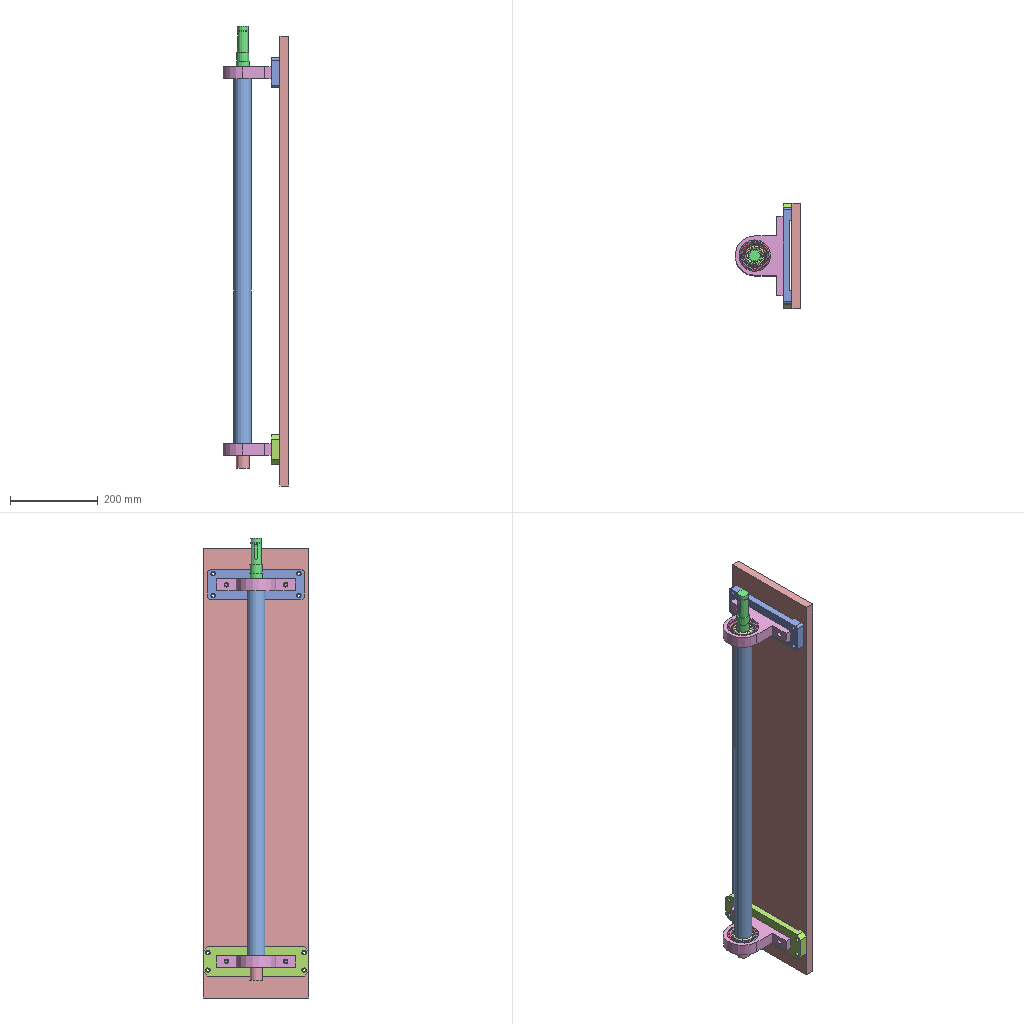Assembly | NX | 5 different items | 7 placed | box 149 x 240 x 1050 mm
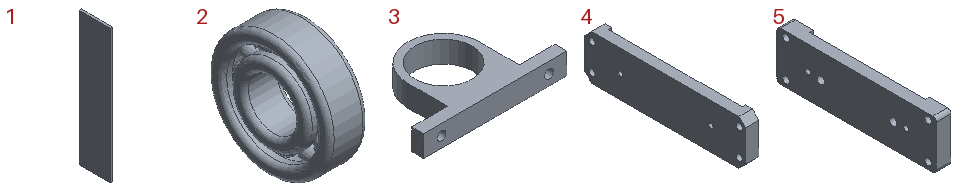Parts list (item | quantity | size | volume | features):
1 | x1 | 20 x 240 x 1027 mm | 4923724 mm3 | features SIMPLE HOLE 8, SYMBOLIC_THREAD 8, LINKED_CURVE 4, DATUM_CSYS 3, SKETCH 2, EXTRUDE 1, HOLE PACKAGE 1, LINKED_FACE 1
2 | x2 | - | 56238 mm3 | features EXTRACT_BODY 12, BLEND 3, DATUM_CSYS 3, SKETCH 2, Container 1, EXTRUDE 1, Geometry Instance 1, Pattern Geometry 1, SHELL 1, SPHERE 1, SUBTRACT 1, SWP104 1
3 | x2 | 180 x 110 x 27 mm | 166653 mm3 | features DATUM_CSYS 5, SKETCH 4, EXTRUDE 3
4 | x1 | 20 x 240 x 67 mm | 244362 mm3 | features SIMPLE HOLE 6, DATUM_CSYS 5, SKETCH 4, EXTRUDE 2, HOLE PACKAGE 2, LINKED_CURVE 2, SYMBOLIC_THREAD 2, CHAMFER 1, LINKED_FACE 1
5 | x1 | 20 x 220 x 67 mm | 232185 mm3 | features SIMPLE HOLE 8, DATUM_CSYS 6, SKETCH 5, HOLE PACKAGE 3, EXTRUDE 2, SYMBOLIC_THREAD 2, BLEND 1, LINKED_CURVE 1, LINKED_FACE 1
Mates (type | each side: item.copy, entity, surface, feature):
Angle | assembly plane | 3.1 face plane Extrude(2)
Angle | 3.1 face plane Extrude(2) | assembly plane
Touch | 3.1 face plane Extrude(2) | 2.1 face plane Revolve(2) | 2 times